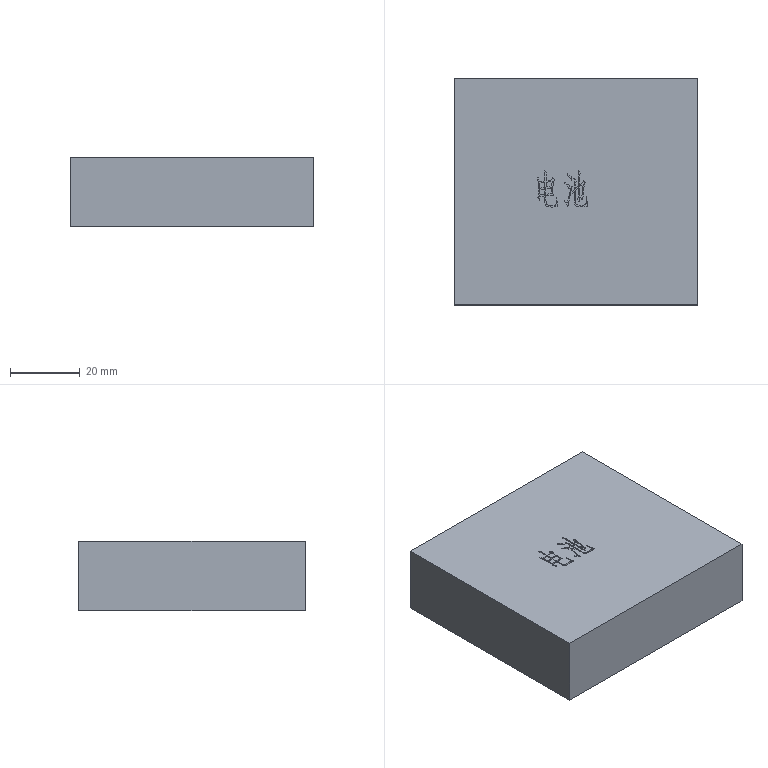Part | SolidWorks | features Extrusion 1, ICE 1 | 1 solid | 192 faces | box 70 x 65 x 20 mm | volume 90986 mm3 | plane 150 | spline 42